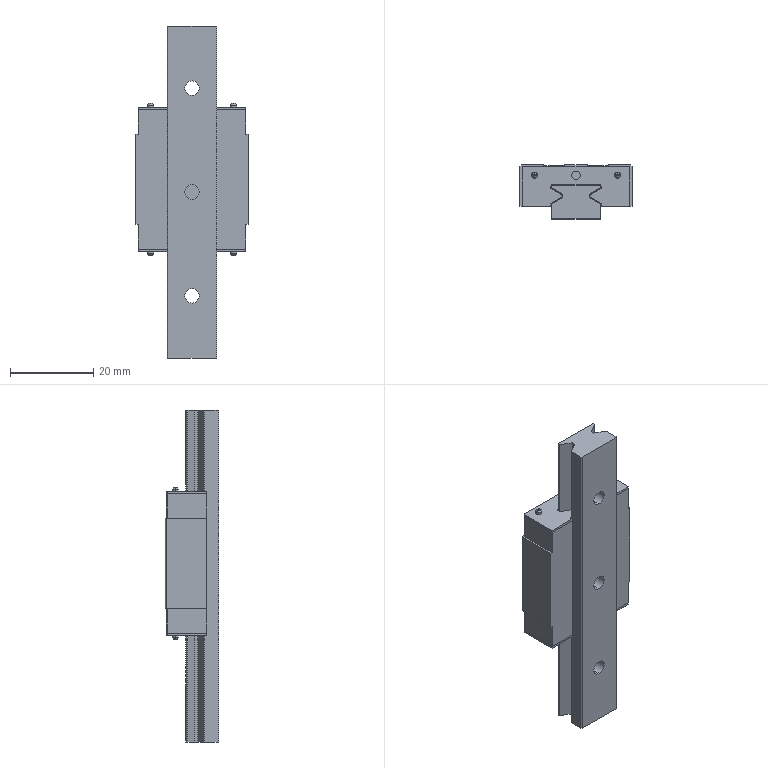Part | SolidWorks | 4 solids | 230 faces | box 27 x 13 x 80 mm | volume 13505 mm3 | plane 190 | cylinder 32 | sphere 8 | commonest cylinder face diameters 1.5 x8 3 x8 3.5 x6 6 x6 2 x4